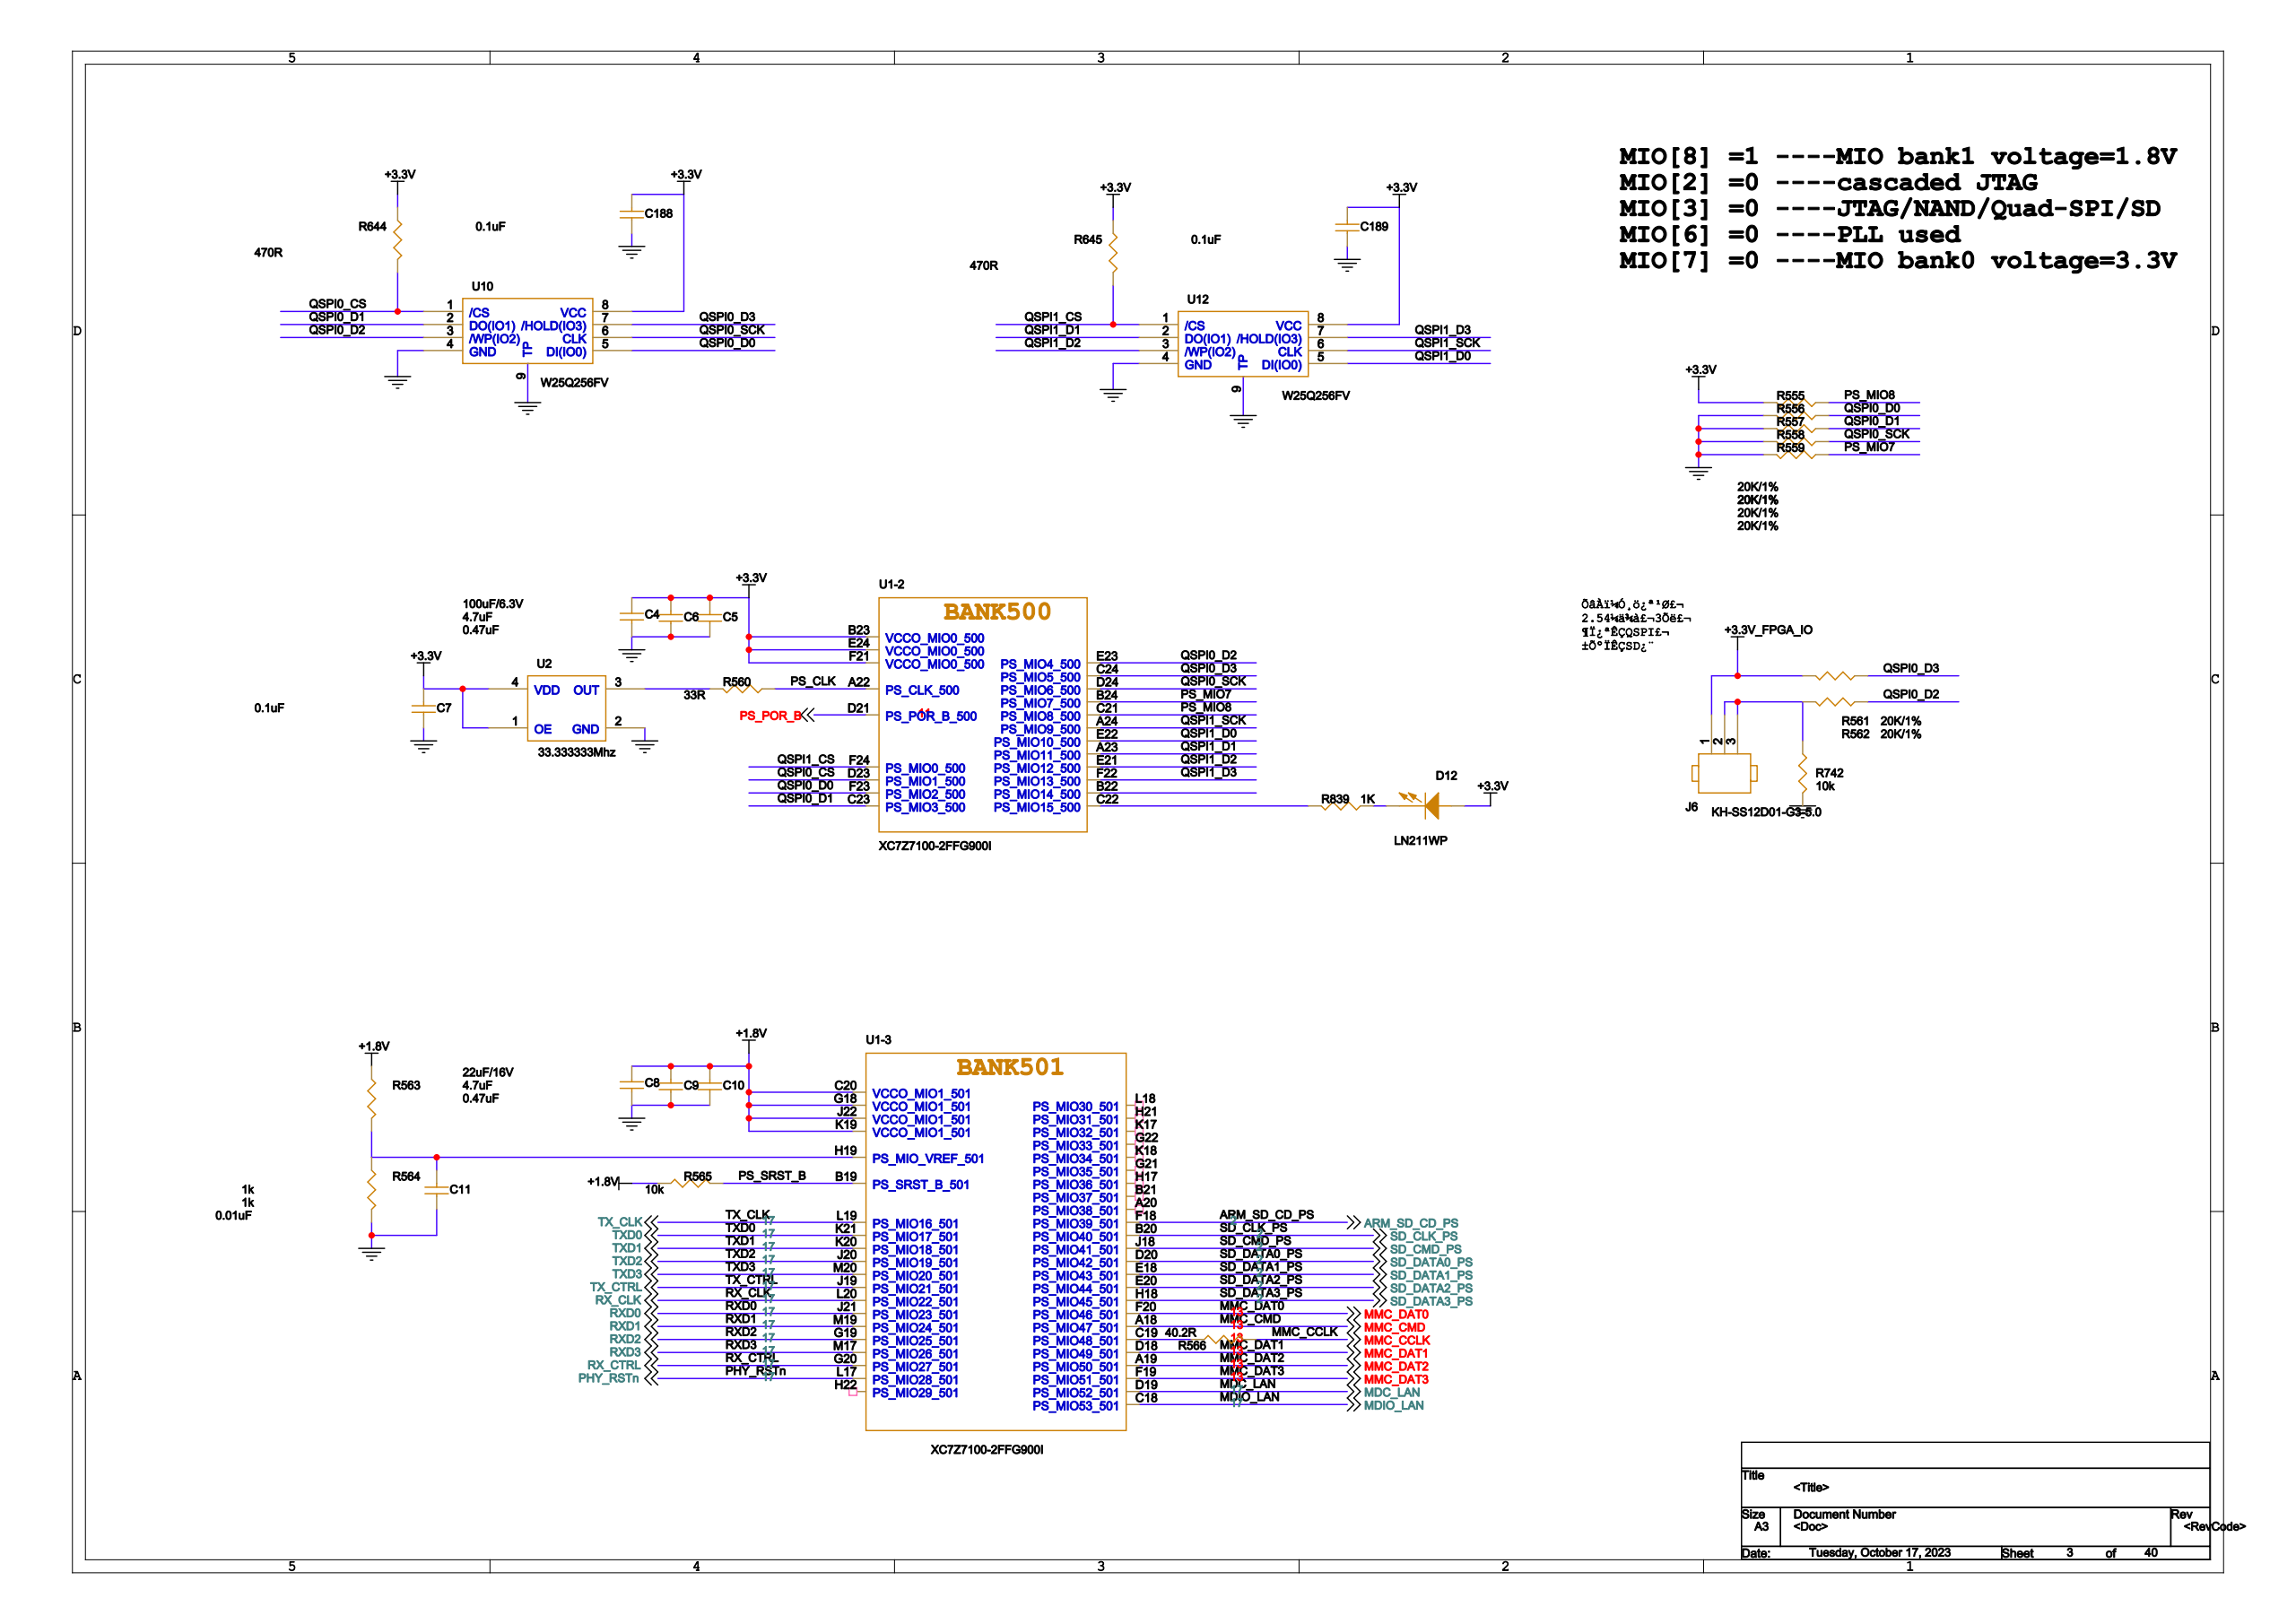Circuit board | Cadence Allegro | 1793 parts | 1223 nets | one sheet of the schematic
Parts on this sheet (reference | value | footprint):
C4 | 100uF/6.3V | 1206
C5 | 0.47uF | C0402
C8 | 22uF/16V | C0603
C9 | 4.7uF | C0402
C10 | 0.47uF | C0402
C11 | 0.01uF | C0402
C18 | 4.7uF | C0402
C188 | 0.1uF | C0402
C189 | 0.1uF | C0402
D12 | LN211WP | D0603
J6 | KH-SS12D01-G3-5.0 | SW-TH_KH-SS12D01-G3-5_0
R555 | 20K/1% | R0402
R556 | 20K/1% | R0402
R557 | 20K/1% | R0402
R558 | 20K/1% | R0402
R559 | 20K/1% | R0402
R560 | 33R | R0402
R561 | 20K/1% | R0402
R562 | 20K/1% | R0402
R563 | 1K | R0402
R564 | 1K | R0402
R565 | 10k | R0402
R566 | 40.2R | R0402
R644 | 470R | R0402
R645 | 470R | R0402
R742 | 10k | R0402
R839 | 1K | R0402
U2 | 33.333Mhz | SMD-25X20
U10 | W25Q256FV | WSON-8X6
U12 | W25Q256FV | WSON-8X6
Nets of these parts (net: part-pin ...):
GND: C4-2 C5-1 C8-2 C9-1 C10-1 C11-1 C18-1 C188-1 C189-1 R556-1 R557-1 R558-1 R559-1 R564-1 R742-1 U2-2 U10-4 U10-9 U12-4 U12-9
+3.3V: C4-1 C5-2 C188-2 C189-2 D12-1 R555-1 R644-2 R645-2 U2-1 U2-4 U10-8 U12-8
+1.8V: C8-1 C9-2 C10-2 R563-2 R565-2
N03232: R560-1 U2-3
N18494: C18-2
PS_MIO8: R555-2
QSPI0_D0: R556-2 U10-5
QSPI0_D1: R557-2 U10-2
QSPI0_SCK: R558-2 U10-6
PS_MIO7: R559-2
+3.3V_FPGA_IO: J6-1 R561-1
QSPI0_D3: R561-2 U10-7
N17324328: J6-2 J6-3 R562-1 R742-2
QSPI0_D2: R562-2 U10-3
PS_CLK: R560-2
MMC_CCLK: R566-1
N07065: R566-2
QSPI0_CS: R644-1 U10-1
QSPI1_CS: R645-1 U12-1
N06094: C11-2 R563-1 R564-2
N16861566: D12-2 R839-2
PS_SRST_B: R565-1
N04461: R839-1
QSPI1_D0: U12-5
QSPI1_D1: U12-2
QSPI1_D2: U12-3
QSPI1_D3: U12-7
QSPI1_SCK: U12-6